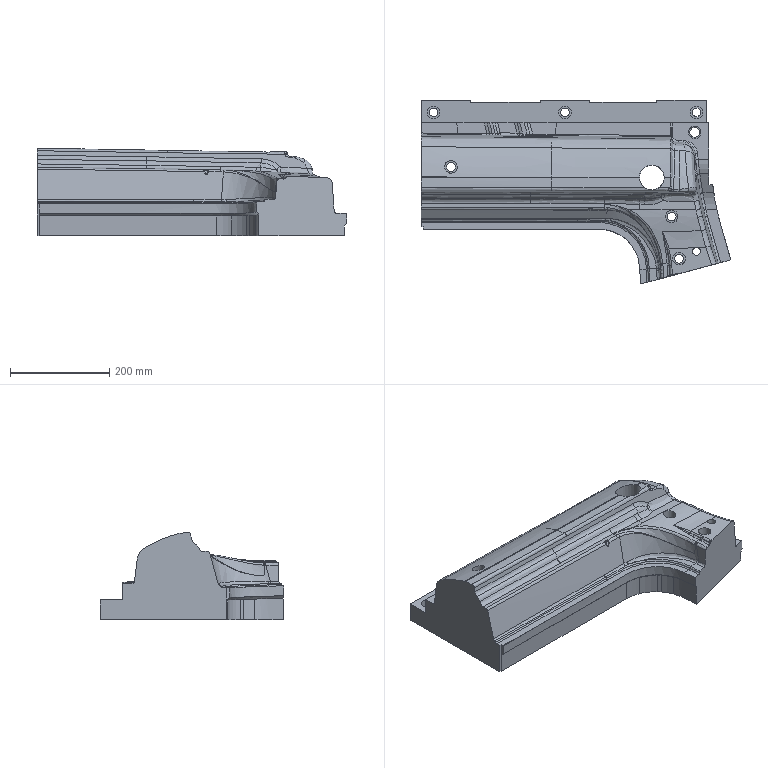Part | NX | features solid 2 | 1 solid | 253 faces | box 624.304 x 370.902 x 175.989 mm | volume 15003985 mm3 | spline 195 | plane 39 | cylinder 19 | commonest cylinder face diameters 17.5 x6 25.5 x6 16 x1 20 x1 25 x1 32 x1